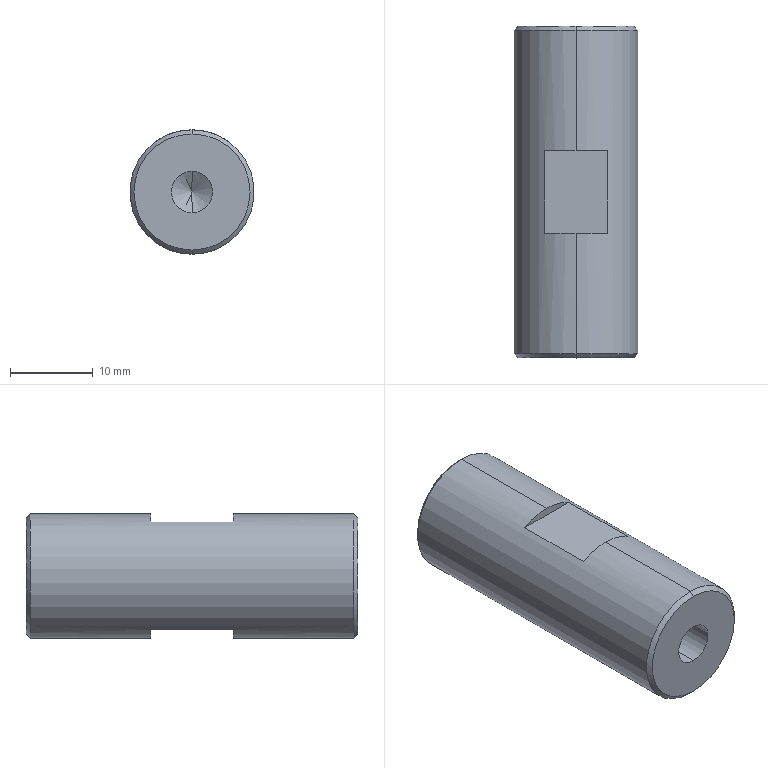Part | STEP file | 11-FG-E02511 | 1 solid | 22 faces | box 15 x 40 x 15 mm | volume 6347 mm3 | cone 8 | plane 8 | cylinder 6 | commonest cylinder face diameters 5 x4 15 x2
STEP:
#1=CARTESIAN_POINT('',(0.,0.,-7.));
#2=VERTEX_POINT('',#1);
#3=CARTESIAN_POINT('',(0.,0.,7.));
#4=VERTEX_POINT('',#3);
#5=CARTESIAN_POINT('',(0.,0.,0.));
#6=DIRECTION('',(0.,-1.,0.));
#7=DIRECTION('',(0.,0.,1.));
#8=AXIS2_PLACEMENT_3D('',#5,#6,#7);
#9=CIRCLE('',#8,7.);
#10=EDGE_CURVE('',#2,#4,#9,.T.);
#11=ORIENTED_EDGE('',*,*,#10,.F.);
#12=CARTESIAN_POINT('',(0.,0.5,-7.5));
#13=VERTEX_POINT('',#12);
#14=CARTESIAN_POINT('',(0.,0.5,-7.5));
#15=DIRECTION('',(0.,0.7071,-0.7071));
#16=VECTOR('',#15,1000.);
#17=LINE('',#14,#16);
#18=EDGE_CURVE('',#2,#13,#17,.T.);
#19=ORIENTED_EDGE('',*,*,#18,.T.);
#20=CARTESIAN_POINT('',(0.,0.5,7.5));
#21=VERTEX_POINT('',#20);
#22=CARTESIAN_POINT('',(0.,0.5,0.));
#23=DIRECTION('',(0.,1.,0.));
#24=DIRECTION('',(0.,0.,1.));
#25=AXIS2_PLACEMENT_3D('',#22,#23,#24);
#26=CIRCLE('',#25,7.5);
#27=EDGE_CURVE('',#21,#13,#26,.T.);
#28=ORIENTED_EDGE('',*,*,#27,.F.);
#29=CARTESIAN_POINT('',(0.,0.5,7.5));
#30=DIRECTION('',(0.,0.7071,0.7071));
#31=VECTOR('',#30,1000.);
#32=LINE('',#29,#31);
#33=EDGE_CURVE('',#4,#21,#32,.T.);
#34=ORIENTED_EDGE('',*,*,#33,.F.);
#35=EDGE_LOOP('',(#11,#19,#28,#34));
#36=FACE_OUTER_BOUND('',#35,.T.);
#37=CARTESIAN_POINT('',(0.,0.5,0.));
#38=DIRECTION('',(0.,1.,0.));
#39=DIRECTION('',(0.,0.,1.));
#40=AXIS2_PLACEMENT_3D('',#37,#38,#39);
#41=CONICAL_SURFACE('',#40,7.5,0.7854);
#42=ADVANCED_FACE('',(#36),#41,.T.);
#43=CARTESIAN_POINT('',(0.,40.,7.));
#44=VERTEX_POINT('',#43);
#45=CARTESIAN_POINT('',(0.,40.,-7.));
#46=VERTEX_POINT('',#45);
#47=CARTESIAN_POINT('',(0.,40.,0.));
#48=DIRECTION('',(0.,1.,0.));
#49=DIRECTION('',(0.,0.,1.));
#50=AXIS2_PLACEMENT_3D('',#47,#48,#49);
#51=CIRCLE('',#50,7.);
#52=EDGE_CURVE('',#44,#46,#51,.T.);
#53=ORIENTED_EDGE('',*,*,#52,.F.);
#54=CARTESIAN_POINT('',(0.,39.5,7.5));
#55=VERTEX_POINT('',#54);
#56=CARTESIAN_POINT('',(0.,40.,7.));
#57=DIRECTION('',(0.,-0.7071,0.7071));
#58=VECTOR('',#57,1000.);
#59=LINE('',#56,#58);
#60=EDGE_CURVE('',#44,#55,#59,.T.);
#61=ORIENTED_EDGE('',*,*,#60,.T.);
#62=CARTESIAN_POINT('',(0.,39.5,-7.5));
#63=VERTEX_POINT('',#62);
#64=CARTESIAN_POINT('',(0.,39.5,0.));
#65=DIRECTION('',(0.,-1.,0.));
#66=DIRECTION('',(0.,0.,1.));
#67=AXIS2_PLACEMENT_3D('',#64,#65,#66);
#68=CIRCLE('',#67,7.5);
#69=EDGE_CURVE('',#63,#55,#68,.T.);
#70=ORIENTED_EDGE('',*,*,#69,.F.);
#71=CARTESIAN_POINT('',(0.,40.,-7.));
#72=DIRECTION('',(0.,-0.7071,-0.7071));
#73=VECTOR('',#72,1000.);
#74=LINE('',#71,#73);
#75=EDGE_CURVE('',#46,#63,#74,.T.);
#76=ORIENTED_EDGE('',*,*,#75,.F.);
#77=EDGE_LOOP('',(#53,#61,#70,#76));
#78=FACE_OUTER_BOUND('',#77,.T.);
#79=CARTESIAN_POINT('',(0.,40.,0.));
#80=DIRECTION('',(0.,-1.,0.));
#81=DIRECTION('',(0.,0.,-1.));
#82=AXIS2_PLACEMENT_3D('',#79,#80,#81);
#83=CONICAL_SURFACE('',#82,7.,0.7854);
#84=ADVANCED_FACE('',(#78),#83,.T.);
#85=CARTESIAN_POINT('',(0.,25.,-2.5));
#86=VERTEX_POINT('',#85);
#87=CARTESIAN_POINT('',(0.,25.,2.5));
#88=VERTEX_POINT('',#87);
#89=CARTESIAN_POINT('',(0.,25.,0.));
#90=DIRECTION('',(0.,1.,0.));
#91=DIRECTION('',(0.,0.,1.));
#92=AXIS2_PLACEMENT_3D('',#89,#90,#91);
#93=CIRCLE('',#92,2.5);
#94=EDGE_CURVE('',#86,#88,#93,.T.);
#95=ORIENTED_EDGE('',*,*,#94,.F.);
#96=CARTESIAN_POINT('',(0.,40.,-2.5));
#97=VERTEX_POINT('',#96);
#98=CARTESIAN_POINT('',(0.,40.,-2.5));
#99=DIRECTION('',(0.,1.,0.));
#100=VECTOR('',#99,1000.);
#101=LINE('',#98,#100);
#102=EDGE_CURVE('',#86,#97,#101,.T.);
#103=ORIENTED_EDGE('',*,*,#102,.T.);
#104=CARTESIAN_POINT('',(0.,40.,2.5));
#105=VERTEX_POINT('',#104);
#106=CARTESIAN_POINT('',(0.,40.,0.));
#107=DIRECTION('',(0.,1.,0.));
#108=DIRECTION('',(0.,0.,1.));
#109=AXIS2_PLACEMENT_3D('',#106,#107,#108);
#110=CIRCLE('',#109,2.5);
#111=EDGE_CURVE('',#97,#105,#110,.T.);
#112=ORIENTED_EDGE('',*,*,#111,.T.);
#113=CARTESIAN_POINT('',(0.,40.,2.5));
#114=DIRECTION('',(0.,1.,0.));
#115=VECTOR('',#114,1000.);
#116=LINE('',#113,#115);
#117=EDGE_CURVE('',#88,#105,#116,.T.);
#118=ORIENTED_EDGE('',*,*,#117,.F.);
#119=EDGE_LOOP('',(#95,#103,#112,#118));
#120=FACE_OUTER_BOUND('',#119,.T.);
#121=CARTESIAN_POINT('',(0.,40.,0.));
#122=DIRECTION('',(0.,1.,0.));
#123=DIRECTION('',(0.,0.,1.));
#124=AXIS2_PLACEMENT_3D('',#121,#122,#123);
#125=CYLINDRICAL_SURFACE('',#124,2.5);
#126=ADVANCED_FACE('',(#120),#125,.F.);
#127=CARTESIAN_POINT('',(0.,23.498,0.));
#128=VERTEX_POINT('',#127);
#129=CARTESIAN_POINT('',(0.,25.,2.5));
#130=DIRECTION('',(0.,0.515,0.8572));
#131=VECTOR('',#130,1000.);
#132=LINE('',#129,#131);
#133=EDGE_CURVE('',#128,#88,#132,.T.);
#134=ORIENTED_EDGE('',*,*,#133,.F.);
#135=CARTESIAN_POINT('',(0.,25.,-2.5));
#136=DIRECTION('',(0.,0.515,-0.8572));
#137=VECTOR('',#136,1000.);
#138=LINE('',#135,#137);
#139=EDGE_CURVE('',#128,#86,#138,.T.);
#140=ORIENTED_EDGE('',*,*,#139,.T.);
#141=ORIENTED_EDGE('',*,*,#94,.T.);
#142=EDGE_LOOP('',(#134,#140,#141));
#143=FACE_OUTER_BOUND('',#142,.T.);
#144=CARTESIAN_POINT('',(0.,25.,0.));
#145=DIRECTION('',(0.,1.,0.));
#146=DIRECTION('',(0.,0.,1.));
#147=AXIS2_PLACEMENT_3D('',#144,#145,#146);
#148=CONICAL_SURFACE('',#147,2.5,1.03);
#149=ADVANCED_FACE('',(#143),#148,.F.);
#150=CARTESIAN_POINT('',(0.,15.,2.5));
#151=VERTEX_POINT('',#150);
#152=CARTESIAN_POINT('',(0.,15.,-2.5));
#153=VERTEX_POINT('',#152);
#154=CARTESIAN_POINT('',(0.,15.,0.));
#155=DIRECTION('',(0.,-1.,0.));
#156=DIRECTION('',(0.,0.,-1.));
#157=AXIS2_PLACEMENT_3D('',#154,#155,#156);
#158=CIRCLE('',#157,2.5);
#159=EDGE_CURVE('',#151,#153,#158,.T.);
#160=ORIENTED_EDGE('',*,*,#159,.F.);
#161=CARTESIAN_POINT('',(0.,0.,2.5));
#162=VERTEX_POINT('',#161);
#163=CARTESIAN_POINT('',(0.,0.,2.5));
#164=DIRECTION('',(0.,-1.,0.));
#165=VECTOR('',#164,1000.);
#166=LINE('',#163,#165);
#167=EDGE_CURVE('',#151,#162,#166,.T.);
#168=ORIENTED_EDGE('',*,*,#167,.T.);
#169=CARTESIAN_POINT('',(0.,0.,-2.5));
#170=VERTEX_POINT('',#169);
#171=CARTESIAN_POINT('',(0.,0.,0.));
#172=DIRECTION('',(0.,-1.,0.));
#173=DIRECTION('',(0.,0.,-1.));
#174=AXIS2_PLACEMENT_3D('',#171,#172,#173);
#175=CIRCLE('',#174,2.5);
#176=EDGE_CURVE('',#162,#170,#175,.T.);
#177=ORIENTED_EDGE('',*,*,#176,.T.);
#178=CARTESIAN_POINT('',(0.,0.,-2.5));
#179=DIRECTION('',(0.,-1.,0.));
#180=VECTOR('',#179,1000.);
#181=LINE('',#178,#180);
#182=EDGE_CURVE('',#153,#170,#181,.T.);
#183=ORIENTED_EDGE('',*,*,#182,.F.);
#184=EDGE_LOOP('',(#160,#168,#177,#183));
#185=FACE_OUTER_BOUND('',#184,.T.);
#186=CARTESIAN_POINT('',(0.,0.,0.));
#187=DIRECTION('',(0.,-1.,0.));
#188=DIRECTION('',(0.,0.,-1.));
#189=AXIS2_PLACEMENT_3D('',#186,#187,#188);
#190=CYLINDRICAL_SURFACE('',#189,2.5);
#191=ADVANCED_FACE('',(#185),#190,.F.);
#192=CARTESIAN_POINT('',(0.,16.502,0.));
#193=VERTEX_POINT('',#192);
#194=CARTESIAN_POINT('',(0.,15.,-2.5));
#195=DIRECTION('',(0.,-0.515,-0.8572));
#196=VECTOR('',#195,1000.);
#197=LINE('',#194,#196);
#198=EDGE_CURVE('',#193,#153,#197,.T.);
#199=ORIENTED_EDGE('',*,*,#198,.F.);
#200=CARTESIAN_POINT('',(0.,15.,2.5));
#201=DIRECTION('',(0.,-0.515,0.8572));
#202=VECTOR('',#201,1000.);
#203=LINE('',#200,#202);
#204=EDGE_CURVE('',#193,#151,#203,.T.);
#205=ORIENTED_EDGE('',*,*,#204,.T.);
#206=ORIENTED_EDGE('',*,*,#159,.T.);
#207=EDGE_LOOP('',(#199,#205,#206));
#208=FACE_OUTER_BOUND('',#207,.T.);
#209=CARTESIAN_POINT('',(0.,15.,0.));
#210=DIRECTION('',(0.,-1.,0.));
#211=DIRECTION('',(0.,0.,-1.));
#212=AXIS2_PLACEMENT_3D('',#209,#210,#211);
#213=CONICAL_SURFACE('',#212,2.5,1.03);
#214=ADVANCED_FACE('',(#208),#213,.F.);
#215=ORIENTED_EDGE('',*,*,#69,.T.);
#216=CARTESIAN_POINT('',(0.,25.,7.5));
#217=VERTEX_POINT('',#216);
#218=CARTESIAN_POINT('',(0.,40.,7.5));
#219=DIRECTION('',(0.,-1.,0.));
#220=VECTOR('',#219,1000.);
#221=LINE('',#218,#220);
#222=EDGE_CURVE('',#55,#217,#221,.T.);
#223=ORIENTED_EDGE('',*,*,#222,.T.);
#224=CARTESIAN_POINT('',(3.742,25.,6.5));
#225=VERTEX_POINT('',#224);
#226=CARTESIAN_POINT('',(0.,25.,0.));
#227=DIRECTION('',(0.,1.,0.));
#228=DIRECTION('',(0.,0.,1.));
#229=AXIS2_PLACEMENT_3D('',#226,#227,#228);
#230=CIRCLE('',#229,7.5);
#231=EDGE_CURVE('',#217,#225,#230,.T.);
#232=ORIENTED_EDGE('',*,*,#231,.T.);
#233=CARTESIAN_POINT('',(3.742,15.,6.5));
#234=VERTEX_POINT('',#233);
#235=CARTESIAN_POINT('',(3.742,15.,6.5));
#236=DIRECTION('',(0.,1.,0.));
#237=VECTOR('',#236,1000.);
#238=LINE('',#235,#237);
#239=EDGE_CURVE('',#234,#225,#238,.T.);
#240=ORIENTED_EDGE('',*,*,#239,.F.);
#241=CARTESIAN_POINT('',(0.,15.,7.5));
#242=VERTEX_POINT('',#241);
#243=CARTESIAN_POINT('',(0.,15.,0.));
#244=DIRECTION('',(0.,1.,0.));
#245=DIRECTION('',(0.,0.,1.));
#246=AXIS2_PLACEMENT_3D('',#243,#244,#245);
#247=CIRCLE('',#246,7.5);
#248=EDGE_CURVE('',#242,#234,#247,.T.);
#249=ORIENTED_EDGE('',*,*,#248,.F.);
#250=CARTESIAN_POINT('',(0.,40.,7.5));
#251=DIRECTION('',(0.,-1.,0.));
#252=VECTOR('',#251,1000.);
#253=LINE('',#250,#252);
#254=EDGE_CURVE('',#242,#21,#253,.T.);
#255=ORIENTED_EDGE('',*,*,#254,.T.);
#256=ORIENTED_EDGE('',*,*,#27,.T.);
#257=CARTESIAN_POINT('',(0.,15.,-7.5));
#258=VERTEX_POINT('',#257);
#259=CARTESIAN_POINT('',(0.,40.,-7.5));
#260=DIRECTION('',(0.,-1.,0.));
#261=VECTOR('',#260,1000.);
#262=LINE('',#259,#261);
#263=EDGE_CURVE('',#258,#13,#262,.T.);
#264=ORIENTED_EDGE('',*,*,#263,.F.);
#265=CARTESIAN_POINT('',(3.742,15.,-6.5));
#266=VERTEX_POINT('',#265);
#267=CARTESIAN_POINT('',(0.,15.,0.));
#268=DIRECTION('',(0.,1.,0.));
#269=DIRECTION('',(0.,0.,1.));
#270=AXIS2_PLACEMENT_3D('',#267,#268,#269);
#271=CIRCLE('',#270,7.5);
#272=EDGE_CURVE('',#266,#258,#271,.T.);
#273=ORIENTED_EDGE('',*,*,#272,.F.);
#274=CARTESIAN_POINT('',(3.742,25.,-6.5));
#275=VERTEX_POINT('',#274);
#276=CARTESIAN_POINT('',(3.742,15.,-6.5));
#277=DIRECTION('',(0.,1.,0.));
#278=VECTOR('',#277,1000.);
#279=LINE('',#276,#278);
#280=EDGE_CURVE('',#266,#275,#279,.T.);
#281=ORIENTED_EDGE('',*,*,#280,.T.);
#282=CARTESIAN_POINT('',(0.,25.,-7.5));
#283=VERTEX_POINT('',#282);
#284=CARTESIAN_POINT('',(0.,25.,0.));
#285=DIRECTION('',(0.,1.,0.));
#286=DIRECTION('',(0.,0.,1.));
#287=AXIS2_PLACEMENT_3D('',#284,#285,#286);
#288=CIRCLE('',#287,7.5);
#289=EDGE_CURVE('',#275,#283,#288,.T.);
#290=ORIENTED_EDGE('',*,*,#289,.T.);
#291=CARTESIAN_POINT('',(0.,40.,-7.5));
#292=DIRECTION('',(0.,-1.,0.));
#293=VECTOR('',#292,1000.);
#294=LINE('',#291,#293);
#295=EDGE_CURVE('',#63,#283,#294,.T.);
#296=ORIENTED_EDGE('',*,*,#295,.F.);
#297=EDGE_LOOP('',(#215,#223,#232,#240,#249,#255,#256,#264,#273,#281,#290,#296));
#298=FACE_OUTER_BOUND('',#297,.T.);
#299=CARTESIAN_POINT('',(0.,40.,0.));
#300=DIRECTION('',(0.,-1.,0.));
#301=DIRECTION('',(0.,0.,-1.));
#302=AXIS2_PLACEMENT_3D('',#299,#300,#301);
#303=CYLINDRICAL_SURFACE('',#302,7.5);
#304=ADVANCED_FACE('',(#298),#303,.T.);
#305=ORIENTED_EDGE('',*,*,#222,.F.);
#306=CARTESIAN_POINT('',(0.,39.5,0.));
#307=DIRECTION('',(0.,-1.,0.));
#308=DIRECTION('',(0.,0.,1.));
#309=AXIS2_PLACEMENT_3D('',#306,#307,#308);
#310=CIRCLE('',#309,7.5);
#311=EDGE_CURVE('',#55,#63,#310,.T.);
#312=ORIENTED_EDGE('',*,*,#311,.T.);
#313=ORIENTED_EDGE('',*,*,#295,.T.);
#314=CARTESIAN_POINT('',(-3.742,25.,-6.5));
#315=VERTEX_POINT('',#314);
#316=CARTESIAN_POINT('',(0.,25.,0.));
#317=DIRECTION('',(0.,1.,0.));
#318=DIRECTION('',(0.,0.,1.));
#319=AXIS2_PLACEMENT_3D('',#316,#317,#318);
#320=CIRCLE('',#319,7.5);
#321=EDGE_CURVE('',#283,#315,#320,.T.);
#322=ORIENTED_EDGE('',*,*,#321,.T.);
#323=CARTESIAN_POINT('',(-3.742,15.,-6.5));
#324=VERTEX_POINT('',#323);
#325=CARTESIAN_POINT('',(-3.742,15.,-6.5));
#326=DIRECTION('',(0.,1.,0.));
#327=VECTOR('',#326,1000.);
#328=LINE('',#325,#327);
#329=EDGE_CURVE('',#324,#315,#328,.T.);
#330=ORIENTED_EDGE('',*,*,#329,.F.);
#331=CARTESIAN_POINT('',(0.,15.,0.));
#332=DIRECTION('',(0.,1.,0.));
#333=DIRECTION('',(0.,0.,1.));
#334=AXIS2_PLACEMENT_3D('',#331,#332,#333);
#335=CIRCLE('',#334,7.5);
#336=EDGE_CURVE('',#258,#324,#335,.T.);
#337=ORIENTED_EDGE('',*,*,#336,.F.);
#338=ORIENTED_EDGE('',*,*,#263,.T.);
#339=CARTESIAN_POINT('',(0.,0.5,0.));
#340=DIRECTION('',(0.,1.,0.));
#341=DIRECTION('',(0.,0.,1.));
#342=AXIS2_PLACEMENT_3D('',#339,#340,#341);
#343=CIRCLE('',#342,7.5);
#344=EDGE_CURVE('',#13,#21,#343,.T.);
#345=ORIENTED_EDGE('',*,*,#344,.T.);
#346=ORIENTED_EDGE('',*,*,#254,.F.);
#347=CARTESIAN_POINT('',(-3.742,15.,6.5));
#348=VERTEX_POINT('',#347);
#349=CARTESIAN_POINT('',(0.,15.,0.));
#350=DIRECTION('',(0.,1.,0.));
#351=DIRECTION('',(0.,0.,1.));
#352=AXIS2_PLACEMENT_3D('',#349,#350,#351);
#353=CIRCLE('',#352,7.5);
#354=EDGE_CURVE('',#348,#242,#353,.T.);
#355=ORIENTED_EDGE('',*,*,#354,.F.);
#356=CARTESIAN_POINT('',(-3.742,25.,6.5));
#357=VERTEX_POINT('',#356);
#358=CARTESIAN_POINT('',(-3.742,15.,6.5));
#359=DIRECTION('',(0.,1.,0.));
#360=VECTOR('',#359,1000.);
#361=LINE('',#358,#360);
#362=EDGE_CURVE('',#348,#357,#361,.T.);
#363=ORIENTED_EDGE('',*,*,#362,.T.);
#364=CARTESIAN_POINT('',(0.,25.,0.));
#365=DIRECTION('',(0.,1.,0.));
#366=DIRECTION('',(0.,0.,1.));
#367=AXIS2_PLACEMENT_3D('',#364,#365,#366);
#368=CIRCLE('',#367,7.5);
#369=EDGE_CURVE('',#357,#217,#368,.T.);
#370=ORIENTED_EDGE('',*,*,#369,.T.);
#371=EDGE_LOOP('',(#305,#312,#313,#322,#330,#337,#338,#345,#346,#355,#363,#370));
#372=FACE_OUTER_BOUND('',#371,.T.);
#373=CARTESIAN_POINT('',(0.,40.,0.));
#374=DIRECTION('',(0.,-1.,0.));
#375=DIRECTION('',(0.,0.,-1.));
#376=AXIS2_PLACEMENT_3D('',#373,#374,#375);
#377=CYLINDRICAL_SURFACE('',#376,7.5);
#378=ADVANCED_FACE('',(#372),#377,.T.);
#379=CARTESIAN_POINT('',(0.,40.,0.));
#380=DIRECTION('',(0.,1.,0.));
#381=DIRECTION('',(0.,0.,1.));
#382=AXIS2_PLACEMENT_3D('',#379,#380,#381);
#383=CIRCLE('',#382,7.);
#384=EDGE_CURVE('',#46,#44,#383,.T.);
#385=ORIENTED_EDGE('',*,*,#384,.T.);
#386=ORIENTED_EDGE('',*,*,#52,.T.);
#387=EDGE_LOOP('',(#385,#386));
#388=FACE_OUTER_BOUND('',#387,.T.);
#389=CARTESIAN_POINT('',(0.,40.,0.));
#390=DIRECTION('',(0.,1.,0.));
#391=DIRECTION('',(0.,0.,1.));
#392=AXIS2_PLACEMENT_3D('',#389,#390,#391);
#393=CIRCLE('',#392,2.5);
#394=EDGE_CURVE('',#105,#97,#393,.T.);
#395=ORIENTED_EDGE('',*,*,#394,.F.);
#396=ORIENTED_EDGE('',*,*,#111,.F.);
#397=EDGE_LOOP('',(#395,#396));
#398=FACE_BOUND('',#397,.T.);
#399=CARTESIAN_POINT('',(0.,40.,0.));
#400=DIRECTION('',(0.,1.,0.));
#401=DIRECTION('',(0.,0.,1.));
#402=AXIS2_PLACEMENT_3D('',#399,#400,#401);
#403=PLANE('',#402);
#404=ADVANCED_FACE('',(#388,#398),#403,.T.);
#405=CARTESIAN_POINT('',(0.,0.,0.));
#406=DIRECTION('',(0.,-1.,0.));
#407=DIRECTION('',(0.,0.,1.));
#408=AXIS2_PLACEMENT_3D('',#405,#406,#407);
#409=CIRCLE('',#408,7.);
#410=EDGE_CURVE('',#4,#2,#409,.T.);
#411=ORIENTED_EDGE('',*,*,#410,.T.);
#412=ORIENTED_EDGE('',*,*,#10,.T.);
#413=EDGE_LOOP('',(#411,#412));
#414=FACE_OUTER_BOUND('',#413,.T.);
#415=CARTESIAN_POINT('',(0.,0.,0.));
#416=DIRECTION('',(0.,-1.,0.));
#417=DIRECTION('',(0.,0.,-1.));
#418=AXIS2_PLACEMENT_3D('',#415,#416,#417);
#419=CIRCLE('',#418,2.5);
#420=EDGE_CURVE('',#170,#162,#419,.T.);
#421=ORIENTED_EDGE('',*,*,#420,.F.);
#422=ORIENTED_EDGE('',*,*,#176,.F.);
#423=EDGE_LOOP('',(#421,#422));
#424=FACE_BOUND('',#423,.T.);
#425=CARTESIAN_POINT('',(0.,0.,0.));
#426=DIRECTION('',(0.,1.,0.));
#427=DIRECTION('',(0.,0.,1.));
#428=AXIS2_PLACEMENT_3D('',#425,#426,#427);
#429=PLANE('',#428);
#430=ADVANCED_FACE('',(#414,#424),#429,.F.);
#431=ORIENTED_EDGE('',*,*,#204,.F.);
#432=ORIENTED_EDGE('',*,*,#198,.T.);
#433=CARTESIAN_POINT('',(0.,15.,0.));
#434=DIRECTION('',(0.,-1.,0.));
#435=DIRECTION('',(0.,0.,-1.));
#436=AXIS2_PLACEMENT_3D('',#433,#434,#435);
#437=CIRCLE('',#436,2.5);
#438=EDGE_CURVE('',#153,#151,#437,.T.);
#439=ORIENTED_EDGE('',*,*,#438,.T.);
#440=EDGE_LOOP('',(#431,#432,#439));
#441=FACE_OUTER_BOUND('',#440,.T.);
#442=CARTESIAN_POINT('',(0.,15.,0.));
#443=DIRECTION('',(0.,-1.,0.));
#444=DIRECTION('',(0.,0.,-1.));
#445=AXIS2_PLACEMENT_3D('',#442,#443,#444);
#446=CONICAL_SURFACE('',#445,2.5,1.03);
#447=ADVANCED_FACE('',(#441),#446,.F.);
#448=ORIENTED_EDGE('',*,*,#167,.F.);
#449=ORIENTED_EDGE('',*,*,#438,.F.);
#450=ORIENTED_EDGE('',*,*,#182,.T.);
#451=ORIENTED_EDGE('',*,*,#420,.T.);
#452=EDGE_LOOP('',(#448,#449,#450,#451));
#453=FACE_OUTER_BOUND('',#452,.T.);
#454=CARTESIAN_POINT('',(0.,0.,0.));
#455=DIRECTION('',(0.,-1.,0.));
#456=DIRECTION('',(0.,0.,-1.));
#457=AXIS2_PLACEMENT_3D('',#454,#455,#456);
#458=CYLINDRICAL_SURFACE('',#457,2.5);
#459=ADVANCED_FACE('',(#453),#458,.F.);
#460=ORIENTED_EDGE('',*,*,#139,.F.);
#461=ORIENTED_EDGE('',*,*,#133,.T.);
#462=CARTESIAN_POINT('',(0.,25.,0.));
#463=DIRECTION('',(0.,1.,0.));
#464=DIRECTION('',(0.,0.,1.));
#465=AXIS2_PLACEMENT_3D('',#462,#463,#464);
#466=CIRCLE('',#465,2.5);
#467=EDGE_CURVE('',#88,#86,#466,.T.);
#468=ORIENTED_EDGE('',*,*,#467,.T.);
#469=EDGE_LOOP('',(#460,#461,#468));
#470=FACE_OUTER_BOUND('',#469,.T.);
#471=CARTESIAN_POINT('',(0.,25.,0.));
#472=DIRECTION('',(0.,1.,0.));
#473=DIRECTION('',(0.,0.,1.));
#474=AXIS2_PLACEMENT_3D('',#471,#472,#473);
#475=CONICAL_SURFACE('',#474,2.5,1.03);
#476=ADVANCED_FACE('',(#470),#475,.F.);
#477=ORIENTED_EDGE('',*,*,#102,.F.);
#478=ORIENTED_EDGE('',*,*,#467,.F.);
#479=ORIENTED_EDGE('',*,*,#117,.T.);
#480=ORIENTED_EDGE('',*,*,#394,.T.);
#481=EDGE_LOOP('',(#477,#478,#479,#480));
#482=FACE_OUTER_BOUND('',#481,.T.);
#483=CARTESIAN_POINT('',(0.,40.,0.));
#484=DIRECTION('',(0.,1.,0.));
#485=DIRECTION('',(0.,0.,1.));
#486=AXIS2_PLACEMENT_3D('',#483,#484,#485);
#487=CYLINDRICAL_SURFACE('',#486,2.5);
#488=ADVANCED_FACE('',(#482),#487,.F.);
#489=ORIENTED_EDGE('',*,*,#60,.F.);
#490=ORIENTED_EDGE('',*,*,#384,.F.);
#491=ORIENTED_EDGE('',*,*,#75,.T.);
#492=ORIENTED_EDGE('',*,*,#311,.F.);
#493=EDGE_LOOP('',(#489,#490,#491,#492));
#494=FACE_OUTER_BOUND('',#493,.T.);
#495=CARTESIAN_POINT('',(0.,40.,0.));
#496=DIRECTION('',(0.,-1.,0.));
#497=DIRECTION('',(0.,0.,-1.));
#498=AXIS2_PLACEMENT_3D('',#495,#496,#497);
#499=CONICAL_SURFACE('',#498,7.,0.7854);
#500=ADVANCED_FACE('',(#494),#499,.T.);
#501=ORIENTED_EDGE('',*,*,#18,.F.);
#502=ORIENTED_EDGE('',*,*,#410,.F.);
#503=ORIENTED_EDGE('',*,*,#33,.T.);
#504=ORIENTED_EDGE('',*,*,#344,.F.);
#505=EDGE_LOOP('',(#501,#502,#503,#504));
#506=FACE_OUTER_BOUND('',#505,.T.);
#507=CARTESIAN_POINT('',(0.,0.5,0.));
#508=DIRECTION('',(0.,1.,0.));
#509=DIRECTION('',(0.,0.,1.));
#510=AXIS2_PLACEMENT_3D('',#507,#508,#509);
#511=CONICAL_SURFACE('',#510,7.5,0.7854);
#512=ADVANCED_FACE('',(#506),#511,.T.);
#513=CARTESIAN_POINT('',(-3.742,25.,-6.5));
#514=DIRECTION('',(1.,0.,0.));
#515=VECTOR('',#514,1000.);
#516=LINE('',#513,#515);
#517=EDGE_CURVE('',#315,#275,#516,.T.);
#518=ORIENTED_EDGE('',*,*,#517,.T.);
#519=ORIENTED_EDGE('',*,*,#280,.F.);
#520=CARTESIAN_POINT('',(-3.742,15.,-6.5));
#521=DIRECTION('',(1.,0.,0.));
#522=VECTOR('',#521,1000.);
#523=LINE('',#520,#522);
#524=EDGE_CURVE('',#324,#266,#523,.T.);
#525=ORIENTED_EDGE('',*,*,#524,.F.);
#526=ORIENTED_EDGE('',*,*,#329,.T.);
#527=EDGE_LOOP('',(#518,#519,#525,#526));
#528=FACE_OUTER_BOUND('',#527,.T.);
#529=CARTESIAN_POINT('',(-3.742,15.,-6.5));
#530=DIRECTION('',(0.,0.,1.));
#531=DIRECTION('',(1.,0.,0.));
#532=AXIS2_PLACEMENT_3D('',#529,#530,#531);
#533=PLANE('',#532);
#534=ADVANCED_FACE('',(#528),#533,.F.);
#535=ORIENTED_EDGE('',*,*,#272,.T.);
#536=ORIENTED_EDGE('',*,*,#336,.T.);
#537=ORIENTED_EDGE('',*,*,#524,.T.);
#538=EDGE_LOOP('',(#535,#536,#537));
#539=FACE_OUTER_BOUND('',#538,.T.);
#540=CARTESIAN_POINT('',(0.,15.,0.));
#541=DIRECTION('',(0.,1.,0.));
#542=DIRECTION('',(0.,0.,1.));
#543=AXIS2_PLACEMENT_3D('',#540,#541,#542);
#544=PLANE('',#543);
#545=ADVANCED_FACE('',(#539),#544,.T.);
#546=ORIENTED_EDGE('',*,*,#289,.F.);
#547=ORIENTED_EDGE('',*,*,#517,.F.);
#548=ORIENTED_EDGE('',*,*,#321,.F.);
#549=EDGE_LOOP('',(#546,#547,#548));
#550=FACE_OUTER_BOUND('',#549,.T.);
#551=CARTESIAN_POINT('',(0.,25.,0.));
#552=DIRECTION('',(0.,1.,0.));
#553=DIRECTION('',(0.,0.,1.));
#554=AXIS2_PLACEMENT_3D('',#551,#552,#553);
#555=PLANE('',#554);
#556=ADVANCED_FACE('',(#550),#555,.F.);
#557=CARTESIAN_POINT('',(-3.742,25.,6.5));
#558=DIRECTION('',(-1.,0.,0.));
#559=VECTOR('',#558,1000.);
#560=LINE('',#557,#559);
#561=EDGE_CURVE('',#225,#357,#560,.T.);
#562=ORIENTED_EDGE('',*,*,#561,.T.);
#563=ORIENTED_EDGE('',*,*,#362,.F.);
#564=CARTESIAN_POINT('',(-3.742,15.,6.5));
#565=DIRECTION('',(-1.,0.,0.));
#566=VECTOR('',#565,1000.);
#567=LINE('',#564,#566);
#568=EDGE_CURVE('',#234,#348,#567,.T.);
#569=ORIENTED_EDGE('',*,*,#568,.F.);
#570=ORIENTED_EDGE('',*,*,#239,.T.);
#571=EDGE_LOOP('',(#562,#563,#569,#570));
#572=FACE_OUTER_BOUND('',#571,.T.);
#573=CARTESIAN_POINT('',(-3.742,15.,6.5));
#574=DIRECTION('',(0.,0.,-1.));
#575=DIRECTION('',(-1.,0.,0.));
#576=AXIS2_PLACEMENT_3D('',#573,#574,#575);
#577=PLANE('',#576);
#578=ADVANCED_FACE('',(#572),#577,.F.);
#579=ORIENTED_EDGE('',*,*,#354,.T.);
#580=ORIENTED_EDGE('',*,*,#248,.T.);
#581=ORIENTED_EDGE('',*,*,#568,.T.);
#582=EDGE_LOOP('',(#579,#580,#581));
#583=FACE_OUTER_BOUND('',#582,.T.);
#584=CARTESIAN_POINT('',(0.,15.,0.));
#585=DIRECTION('',(0.,1.,0.));
#586=DIRECTION('',(0.,0.,1.));
#587=AXIS2_PLACEMENT_3D('',#584,#585,#586);
#588=PLANE('',#587);
#589=ADVANCED_FACE('',(#583),#588,.T.);
#590=ORIENTED_EDGE('',*,*,#369,.F.);
#591=ORIENTED_EDGE('',*,*,#561,.F.);
#592=ORIENTED_EDGE('',*,*,#231,.F.);
#593=EDGE_LOOP('',(#590,#591,#592));
#594=FACE_OUTER_BOUND('',#593,.T.);
#595=CARTESIAN_POINT('',(0.,25.,0.));
#596=DIRECTION('',(0.,1.,0.));
#597=DIRECTION('',(0.,0.,1.));
#598=AXIS2_PLACEMENT_3D('',#595,#596,#597);
#599=PLANE('',#598);
#600=ADVANCED_FACE('',(#594),#599,.F.);
#601=CLOSED_SHELL('',(#42,#84,#126,#149,#191,#214,#304,#378,#404,#430,#447,#459,#476,#488,#500,#512,#534,#545,#556,#578,#589,#600));
#602=MANIFOLD_SOLID_BREP('',#601);
#603=CARTESIAN_POINT('',(0.,0.,0.));
#604=DIRECTION('',(0.,0.,1.));
#605=DIRECTION('',(1.,0.,0.));
#606=AXIS2_PLACEMENT_3D('',#603,#604,#605);
#607=(LENGTH_UNIT()NAMED_UNIT(*)SI_UNIT(.MILLI.,.METRE.));
#608=UNCERTAINTY_MEASURE_WITH_UNIT(LENGTH_MEASURE(0.00001),#607,'','');
#609=(NAMED_UNIT(*)PLANE_ANGLE_UNIT()SI_UNIT($,.RADIAN.));
#610=(NAMED_UNIT(*)SI_UNIT($,.STERADIAN.)SOLID_ANGLE_UNIT());
#611=(GEOMETRIC_REPRESENTATION_CONTEXT(3)GLOBAL_UNCERTAINTY_ASSIGNED_CONTEXT((#608))GLOBAL_UNIT_ASSIGNED_CONTEXT((#607,#609,#610))REPRESENTATION_CONTEXT('',''));
#612=ADVANCED_BREP_SHAPE_REPRESENTATION('',(#602,#606),#611);